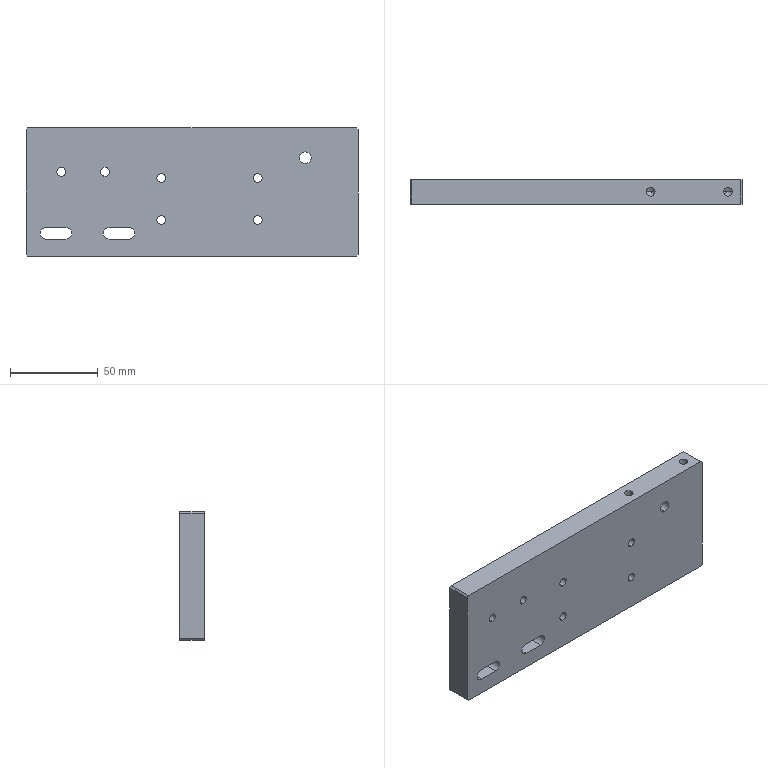Part | SolidWorks | features HoleWzd 5, Chamfer 1, Extrusion 1 | 1 solid | 43 faces | box 189 x 14 x 73 mm | volume 186915 mm3 | cylinder 24 | plane 15 | cone 4 | commonest cylinder face diameters 5 x16 6.6 x6 11 x2
STEP:
#1=CARTESIAN_POINT('',(64.5,0.2,14.));
#2=VERTEX_POINT('',#1);
#3=CARTESIAN_POINT('',(64.5,0.2,25.));
#4=VERTEX_POINT('',#3);
#5=CARTESIAN_POINT('',(64.5,0.2,19.5));
#6=DIRECTION('',(0.,1.,0.));
#7=DIRECTION('',(0.,0.,1.));
#8=AXIS2_PLACEMENT_3D('',#5,#6,#7);
#9=CIRCLE('',#8,5.5);
#10=EDGE_CURVE('',#2,#4,#9,.T.);
#11=ORIENTED_EDGE('',*,*,#10,.F.);
#12=CARTESIAN_POINT('',(64.5,7.,14.));
#13=VERTEX_POINT('',#12);
#14=CARTESIAN_POINT('',(64.5,7.,14.));
#15=DIRECTION('',(0.,1.,0.));
#16=VECTOR('',#15,1000.);
#17=LINE('',#14,#16);
#18=EDGE_CURVE('',#2,#13,#17,.T.);
#19=ORIENTED_EDGE('',*,*,#18,.T.);
#20=CARTESIAN_POINT('',(64.5,7.,25.));
#21=VERTEX_POINT('',#20);
#22=CARTESIAN_POINT('',(64.5,7.,19.5));
#23=DIRECTION('',(0.,1.,0.));
#24=DIRECTION('',(0.,0.,1.));
#25=AXIS2_PLACEMENT_3D('',#22,#23,#24);
#26=CIRCLE('',#25,5.5);
#27=EDGE_CURVE('',#13,#21,#26,.T.);
#28=ORIENTED_EDGE('',*,*,#27,.T.);
#29=CARTESIAN_POINT('',(64.5,7.,25.));
#30=DIRECTION('',(0.,1.,0.));
#31=VECTOR('',#30,1000.);
#32=LINE('',#29,#31);
#33=EDGE_CURVE('',#4,#21,#32,.T.);
#34=ORIENTED_EDGE('',*,*,#33,.F.);
#35=EDGE_LOOP('',(#11,#19,#28,#34));
#36=FACE_OUTER_BOUND('',#35,.T.);
#37=CARTESIAN_POINT('',(64.5,7.,19.5));
#38=DIRECTION('',(0.,1.,0.));
#39=DIRECTION('',(0.,0.,1.));
#40=AXIS2_PLACEMENT_3D('',#37,#38,#39);
#41=CYLINDRICAL_SURFACE('',#40,5.5);
#42=ADVANCED_FACE('',(#36),#41,.F.);
#43=CARTESIAN_POINT('',(64.5,-7.,16.2));
#44=VERTEX_POINT('',#43);
#45=CARTESIAN_POINT('',(64.5,-7.,22.8));
#46=VERTEX_POINT('',#45);
#47=CARTESIAN_POINT('',(64.5,-7.,19.5));
#48=DIRECTION('',(0.,1.,0.));
#49=DIRECTION('',(0.,0.,1.));
#50=AXIS2_PLACEMENT_3D('',#47,#48,#49);
#51=CIRCLE('',#50,3.3);
#52=EDGE_CURVE('',#44,#46,#51,.T.);
#53=ORIENTED_EDGE('',*,*,#52,.F.);
#54=CARTESIAN_POINT('',(64.5,0.2,16.2));
#55=VERTEX_POINT('',#54);
#56=CARTESIAN_POINT('',(64.5,7.,16.2));
#57=DIRECTION('',(0.,1.,0.));
#58=VECTOR('',#57,1000.);
#59=LINE('',#56,#58);
#60=EDGE_CURVE('',#44,#55,#59,.T.);
#61=ORIENTED_EDGE('',*,*,#60,.T.);
#62=CARTESIAN_POINT('',(64.5,0.2,22.8));
#63=VERTEX_POINT('',#62);
#64=CARTESIAN_POINT('',(64.5,0.2,19.5));
#65=DIRECTION('',(0.,1.,0.));
#66=DIRECTION('',(0.,0.,1.));
#67=AXIS2_PLACEMENT_3D('',#64,#65,#66);
#68=CIRCLE('',#67,3.3);
#69=EDGE_CURVE('',#55,#63,#68,.T.);
#70=ORIENTED_EDGE('',*,*,#69,.T.);
#71=CARTESIAN_POINT('',(64.5,7.,22.8));
#72=DIRECTION('',(0.,1.,0.));
#73=VECTOR('',#72,1000.);
#74=LINE('',#71,#73);
#75=EDGE_CURVE('',#46,#63,#74,.T.);
#76=ORIENTED_EDGE('',*,*,#75,.F.);
#77=EDGE_LOOP('',(#53,#61,#70,#76));
#78=FACE_OUTER_BOUND('',#77,.T.);
#79=CARTESIAN_POINT('',(64.5,7.,19.5));
#80=DIRECTION('',(0.,1.,0.));
#81=DIRECTION('',(0.,0.,1.));
#82=AXIS2_PLACEMENT_3D('',#79,#80,#81);
#83=CYLINDRICAL_SURFACE('',#82,3.3);
#84=ADVANCED_FACE('',(#78),#83,.F.);
#85=CARTESIAN_POINT('',(-74.5,-7.,9.));
#86=VERTEX_POINT('',#85);
#87=CARTESIAN_POINT('',(-74.5,-7.,14.));
#88=VERTEX_POINT('',#87);
#89=CARTESIAN_POINT('',(-74.5,-7.,11.5));
#90=DIRECTION('',(0.,1.,0.));
#91=DIRECTION('',(0.,0.,1.));
#92=AXIS2_PLACEMENT_3D('',#89,#90,#91);
#93=CIRCLE('',#92,2.5);
#94=EDGE_CURVE('',#86,#88,#93,.T.);
#95=ORIENTED_EDGE('',*,*,#94,.F.);
#96=CARTESIAN_POINT('',(-74.5,7.,9.));
#97=VERTEX_POINT('',#96);
#98=CARTESIAN_POINT('',(-74.5,7.,9.));
#99=DIRECTION('',(0.,1.,0.));
#100=VECTOR('',#99,1000.);
#101=LINE('',#98,#100);
#102=EDGE_CURVE('',#86,#97,#101,.T.);
#103=ORIENTED_EDGE('',*,*,#102,.T.);
#104=CARTESIAN_POINT('',(-74.5,7.,14.));
#105=VERTEX_POINT('',#104);
#106=CARTESIAN_POINT('',(-74.5,7.,11.5));
#107=DIRECTION('',(0.,1.,0.));
#108=DIRECTION('',(0.,0.,1.));
#109=AXIS2_PLACEMENT_3D('',#106,#107,#108);
#110=CIRCLE('',#109,2.5);
#111=EDGE_CURVE('',#97,#105,#110,.T.);
#112=ORIENTED_EDGE('',*,*,#111,.T.);
#113=CARTESIAN_POINT('',(-74.5,7.,14.));
#114=DIRECTION('',(0.,1.,0.));
#115=VECTOR('',#114,1000.);
#116=LINE('',#113,#115);
#117=EDGE_CURVE('',#88,#105,#116,.T.);
#118=ORIENTED_EDGE('',*,*,#117,.F.);
#119=EDGE_LOOP('',(#95,#103,#112,#118));
#120=FACE_OUTER_BOUND('',#119,.T.);
#121=CARTESIAN_POINT('',(-74.5,7.,11.5));
#122=DIRECTION('',(0.,1.,0.));
#123=DIRECTION('',(0.,0.,1.));
#124=AXIS2_PLACEMENT_3D('',#121,#122,#123);
#125=CYLINDRICAL_SURFACE('',#124,2.5);
#126=ADVANCED_FACE('',(#120),#125,.F.);
#127=CARTESIAN_POINT('',(-49.5,-7.,9.));
#128=VERTEX_POINT('',#127);
#129=CARTESIAN_POINT('',(-49.5,-7.,14.));
#130=VERTEX_POINT('',#129);
#131=CARTESIAN_POINT('',(-49.5,-7.,11.5));
#132=DIRECTION('',(0.,1.,0.));
#133=DIRECTION('',(0.,0.,1.));
#134=AXIS2_PLACEMENT_3D('',#131,#132,#133);
#135=CIRCLE('',#134,2.5);
#136=EDGE_CURVE('',#128,#130,#135,.T.);
#137=ORIENTED_EDGE('',*,*,#136,.F.);
#138=CARTESIAN_POINT('',(-49.5,7.,9.));
#139=VERTEX_POINT('',#138);
#140=CARTESIAN_POINT('',(-49.5,7.,9.));
#141=DIRECTION('',(0.,1.,0.));
#142=VECTOR('',#141,1000.);
#143=LINE('',#140,#142);
#144=EDGE_CURVE('',#128,#139,#143,.T.);
#145=ORIENTED_EDGE('',*,*,#144,.T.);
#146=CARTESIAN_POINT('',(-49.5,7.,14.));
#147=VERTEX_POINT('',#146);
#148=CARTESIAN_POINT('',(-49.5,7.,11.5));
#149=DIRECTION('',(0.,1.,0.));
#150=DIRECTION('',(0.,0.,1.));
#151=AXIS2_PLACEMENT_3D('',#148,#149,#150);
#152=CIRCLE('',#151,2.5);
#153=EDGE_CURVE('',#139,#147,#152,.T.);
#154=ORIENTED_EDGE('',*,*,#153,.T.);
#155=CARTESIAN_POINT('',(-49.5,7.,14.));
#156=DIRECTION('',(0.,1.,0.));
#157=VECTOR('',#156,1000.);
#158=LINE('',#155,#157);
#159=EDGE_CURVE('',#130,#147,#158,.T.);
#160=ORIENTED_EDGE('',*,*,#159,.F.);
#161=EDGE_LOOP('',(#137,#145,#154,#160));
#162=FACE_OUTER_BOUND('',#161,.T.);
#163=CARTESIAN_POINT('',(-49.5,7.,11.5));
#164=DIRECTION('',(0.,1.,0.));
#165=DIRECTION('',(0.,0.,1.));
#166=AXIS2_PLACEMENT_3D('',#163,#164,#165);
#167=CYLINDRICAL_SURFACE('',#166,2.5);
#168=ADVANCED_FACE('',(#162),#167,.F.);
#169=CARTESIAN_POINT('',(-17.5,-7.,-18.5));
#170=VERTEX_POINT('',#169);
#171=CARTESIAN_POINT('',(-17.5,-7.,-13.5));
#172=VERTEX_POINT('',#171);
#173=CARTESIAN_POINT('',(-17.5,-7.,-16.));
#174=DIRECTION('',(0.,1.,0.));
#175=DIRECTION('',(0.,0.,1.));
#176=AXIS2_PLACEMENT_3D('',#173,#174,#175);
#177=CIRCLE('',#176,2.5);
#178=EDGE_CURVE('',#170,#172,#177,.T.);
#179=ORIENTED_EDGE('',*,*,#178,.F.);
#180=CARTESIAN_POINT('',(-17.5,7.,-18.5));
#181=VERTEX_POINT('',#180);
#182=CARTESIAN_POINT('',(-17.5,7.,-18.5));
#183=DIRECTION('',(0.,1.,0.));
#184=VECTOR('',#183,1000.);
#185=LINE('',#182,#184);
#186=EDGE_CURVE('',#170,#181,#185,.T.);
#187=ORIENTED_EDGE('',*,*,#186,.T.);
#188=CARTESIAN_POINT('',(-17.5,7.,-13.5));
#189=VERTEX_POINT('',#188);
#190=CARTESIAN_POINT('',(-17.5,7.,-16.));
#191=DIRECTION('',(0.,1.,0.));
#192=DIRECTION('',(0.,0.,1.));
#193=AXIS2_PLACEMENT_3D('',#190,#191,#192);
#194=CIRCLE('',#193,2.5);
#195=EDGE_CURVE('',#181,#189,#194,.T.);
#196=ORIENTED_EDGE('',*,*,#195,.T.);
#197=CARTESIAN_POINT('',(-17.5,7.,-13.5));
#198=DIRECTION('',(0.,1.,0.));
#199=VECTOR('',#198,1000.);
#200=LINE('',#197,#199);
#201=EDGE_CURVE('',#172,#189,#200,.T.);
#202=ORIENTED_EDGE('',*,*,#201,.F.);
#203=EDGE_LOOP('',(#179,#187,#196,#202));
#204=FACE_OUTER_BOUND('',#203,.T.);
#205=CARTESIAN_POINT('',(-17.5,7.,-16.));
#206=DIRECTION('',(0.,1.,0.));
#207=DIRECTION('',(0.,0.,1.));
#208=AXIS2_PLACEMENT_3D('',#205,#206,#207);
#209=CYLINDRICAL_SURFACE('',#208,2.5);
#210=ADVANCED_FACE('',(#204),#209,.F.);
#211=CARTESIAN_POINT('',(37.5,-7.,5.5));
#212=VERTEX_POINT('',#211);
#213=CARTESIAN_POINT('',(37.5,-7.,10.5));
#214=VERTEX_POINT('',#213);
#215=CARTESIAN_POINT('',(37.5,-7.,8.));
#216=DIRECTION('',(0.,1.,0.));
#217=DIRECTION('',(0.,0.,1.));
#218=AXIS2_PLACEMENT_3D('',#215,#216,#217);
#219=CIRCLE('',#218,2.5);
#220=EDGE_CURVE('',#212,#214,#219,.T.);
#221=ORIENTED_EDGE('',*,*,#220,.F.);
#222=CARTESIAN_POINT('',(37.5,7.,5.5));
#223=VERTEX_POINT('',#222);
#224=CARTESIAN_POINT('',(37.5,7.,5.5));
#225=DIRECTION('',(0.,1.,0.));
#226=VECTOR('',#225,1000.);
#227=LINE('',#224,#226);
#228=EDGE_CURVE('',#212,#223,#227,.T.);
#229=ORIENTED_EDGE('',*,*,#228,.T.);
#230=CARTESIAN_POINT('',(37.5,7.,10.5));
#231=VERTEX_POINT('',#230);
#232=CARTESIAN_POINT('',(37.5,7.,8.));
#233=DIRECTION('',(0.,1.,0.));
#234=DIRECTION('',(0.,0.,1.));
#235=AXIS2_PLACEMENT_3D('',#232,#233,#234);
#236=CIRCLE('',#235,2.5);
#237=EDGE_CURVE('',#223,#231,#236,.T.);
#238=ORIENTED_EDGE('',*,*,#237,.T.);
#239=CARTESIAN_POINT('',(37.5,7.,10.5));
#240=DIRECTION('',(0.,1.,0.));
#241=VECTOR('',#240,1000.);
#242=LINE('',#239,#241);
#243=EDGE_CURVE('',#214,#231,#242,.T.);
#244=ORIENTED_EDGE('',*,*,#243,.F.);
#245=EDGE_LOOP('',(#221,#229,#238,#244));
#246=FACE_OUTER_BOUND('',#245,.T.);
#247=CARTESIAN_POINT('',(37.5,7.,8.));
#248=DIRECTION('',(0.,1.,0.));
#249=DIRECTION('',(0.,0.,1.));
#250=AXIS2_PLACEMENT_3D('',#247,#248,#249);
#251=CYLINDRICAL_SURFACE('',#250,2.5);
#252=ADVANCED_FACE('',(#246),#251,.F.);
#253=CARTESIAN_POINT('',(-17.5,-7.,5.5));
#254=VERTEX_POINT('',#253);
#255=CARTESIAN_POINT('',(-17.5,-7.,10.5));
#256=VERTEX_POINT('',#255);
#257=CARTESIAN_POINT('',(-17.5,-7.,8.));
#258=DIRECTION('',(0.,1.,0.));
#259=DIRECTION('',(0.,0.,1.));
#260=AXIS2_PLACEMENT_3D('',#257,#258,#259);
#261=CIRCLE('',#260,2.5);
#262=EDGE_CURVE('',#254,#256,#261,.T.);
#263=ORIENTED_EDGE('',*,*,#262,.F.);
#264=CARTESIAN_POINT('',(-17.5,7.,5.5));
#265=VERTEX_POINT('',#264);
#266=CARTESIAN_POINT('',(-17.5,7.,5.5));
#267=DIRECTION('',(0.,1.,0.));
#268=VECTOR('',#267,1000.);
#269=LINE('',#266,#268);
#270=EDGE_CURVE('',#254,#265,#269,.T.);
#271=ORIENTED_EDGE('',*,*,#270,.T.);
#272=CARTESIAN_POINT('',(-17.5,7.,10.5));
#273=VERTEX_POINT('',#272);
#274=CARTESIAN_POINT('',(-17.5,7.,8.));
#275=DIRECTION('',(0.,1.,0.));
#276=DIRECTION('',(0.,0.,1.));
#277=AXIS2_PLACEMENT_3D('',#274,#275,#276);
#278=CIRCLE('',#277,2.5);
#279=EDGE_CURVE('',#265,#273,#278,.T.);
#280=ORIENTED_EDGE('',*,*,#279,.T.);
#281=CARTESIAN_POINT('',(-17.5,7.,10.5));
#282=DIRECTION('',(0.,1.,0.));
#283=VECTOR('',#282,1000.);
#284=LINE('',#281,#283);
#285=EDGE_CURVE('',#256,#273,#284,.T.);
#286=ORIENTED_EDGE('',*,*,#285,.F.);
#287=EDGE_LOOP('',(#263,#271,#280,#286));
#288=FACE_OUTER_BOUND('',#287,.T.);
#289=CARTESIAN_POINT('',(-17.5,7.,8.));
#290=DIRECTION('',(0.,1.,0.));
#291=DIRECTION('',(0.,0.,1.));
#292=AXIS2_PLACEMENT_3D('',#289,#290,#291);
#293=CYLINDRICAL_SURFACE('',#292,2.5);
#294=ADVANCED_FACE('',(#288),#293,.F.);
#295=CARTESIAN_POINT('',(37.5,-7.,-18.5));
#296=VERTEX_POINT('',#295);
#297=CARTESIAN_POINT('',(37.5,-7.,-13.5));
#298=VERTEX_POINT('',#297);
#299=CARTESIAN_POINT('',(37.5,-7.,-16.));
#300=DIRECTION('',(0.,1.,0.));
#301=DIRECTION('',(0.,0.,1.));
#302=AXIS2_PLACEMENT_3D('',#299,#300,#301);
#303=CIRCLE('',#302,2.5);
#304=EDGE_CURVE('',#296,#298,#303,.T.);
#305=ORIENTED_EDGE('',*,*,#304,.F.);
#306=CARTESIAN_POINT('',(37.5,7.,-18.5));
#307=VERTEX_POINT('',#306);
#308=CARTESIAN_POINT('',(37.5,7.,-18.5));
#309=DIRECTION('',(0.,1.,0.));
#310=VECTOR('',#309,1000.);
#311=LINE('',#308,#310);
#312=EDGE_CURVE('',#296,#307,#311,.T.);
#313=ORIENTED_EDGE('',*,*,#312,.T.);
#314=CARTESIAN_POINT('',(37.5,7.,-13.5));
#315=VERTEX_POINT('',#314);
#316=CARTESIAN_POINT('',(37.5,7.,-16.));
#317=DIRECTION('',(0.,1.,0.));
#318=DIRECTION('',(0.,0.,1.));
#319=AXIS2_PLACEMENT_3D('',#316,#317,#318);
#320=CIRCLE('',#319,2.5);
#321=EDGE_CURVE('',#307,#315,#320,.T.);
#322=ORIENTED_EDGE('',*,*,#321,.T.);
#323=CARTESIAN_POINT('',(37.5,7.,-13.5));
#324=DIRECTION('',(0.,1.,0.));
#325=VECTOR('',#324,1000.);
#326=LINE('',#323,#325);
#327=EDGE_CURVE('',#298,#315,#326,.T.);
#328=ORIENTED_EDGE('',*,*,#327,.F.);
#329=EDGE_LOOP('',(#305,#313,#322,#328));
#330=FACE_OUTER_BOUND('',#329,.T.);
#331=CARTESIAN_POINT('',(37.5,7.,-16.));
#332=DIRECTION('',(0.,1.,0.));
#333=DIRECTION('',(0.,0.,1.));
#334=AXIS2_PLACEMENT_3D('',#331,#332,#333);
#335=CYLINDRICAL_SURFACE('',#334,2.5);
#336=ADVANCED_FACE('',(#330),#335,.F.);
#337=CARTESIAN_POINT('',(84.,0.,21.5));
#338=VERTEX_POINT('',#337);
#339=CARTESIAN_POINT('',(89.,0.,21.5));
#340=VERTEX_POINT('',#339);
#341=CARTESIAN_POINT('',(86.5,0.,21.5));
#342=DIRECTION('',(0.,0.,1.));
#343=DIRECTION('',(1.,0.,0.));
#344=AXIS2_PLACEMENT_3D('',#341,#342,#343);
#345=CIRCLE('',#344,2.5);
#346=EDGE_CURVE('',#338,#340,#345,.T.);
#347=ORIENTED_EDGE('',*,*,#346,.F.);
#348=CARTESIAN_POINT('',(84.,0.,36.5));
#349=VERTEX_POINT('',#348);
#350=CARTESIAN_POINT('',(84.,0.,36.5));
#351=DIRECTION('',(0.,0.,1.));
#352=VECTOR('',#351,1000.);
#353=LINE('',#350,#352);
#354=EDGE_CURVE('',#338,#349,#353,.T.);
#355=ORIENTED_EDGE('',*,*,#354,.T.);
#356=CARTESIAN_POINT('',(89.,0.,36.5));
#357=VERTEX_POINT('',#356);
#358=CARTESIAN_POINT('',(86.5,0.,36.5));
#359=DIRECTION('',(0.,0.,1.));
#360=DIRECTION('',(1.,0.,0.));
#361=AXIS2_PLACEMENT_3D('',#358,#359,#360);
#362=CIRCLE('',#361,2.5);
#363=EDGE_CURVE('',#349,#357,#362,.T.);
#364=ORIENTED_EDGE('',*,*,#363,.T.);
#365=CARTESIAN_POINT('',(89.,0.,36.5));
#366=DIRECTION('',(0.,0.,1.));
#367=VECTOR('',#366,1000.);
#368=LINE('',#365,#367);
#369=EDGE_CURVE('',#340,#357,#368,.T.);
#370=ORIENTED_EDGE('',*,*,#369,.F.);
#371=EDGE_LOOP('',(#347,#355,#364,#370));
#372=FACE_OUTER_BOUND('',#371,.T.);
#373=CARTESIAN_POINT('',(86.5,0.,36.5));
#374=DIRECTION('',(0.,0.,1.));
#375=DIRECTION('',(1.,0.,0.));
#376=AXIS2_PLACEMENT_3D('',#373,#374,#375);
#377=CYLINDRICAL_SURFACE('',#376,2.5);
#378=ADVANCED_FACE('',(#372),#377,.F.);
#379=CARTESIAN_POINT('',(86.5,0.,19.998));
#380=VERTEX_POINT('',#379);
#381=CARTESIAN_POINT('',(89.,0.,21.5));
#382=DIRECTION('',(0.8572,0.,0.515));
#383=VECTOR('',#382,1000.);
#384=LINE('',#381,#383);
#385=EDGE_CURVE('',#380,#340,#384,.T.);
#386=ORIENTED_EDGE('',*,*,#385,.F.);
#387=CARTESIAN_POINT('',(84.,0.,21.5));
#388=DIRECTION('',(-0.8572,0.,0.515));
#389=VECTOR('',#388,1000.);
#390=LINE('',#387,#389);
#391=EDGE_CURVE('',#380,#338,#390,.T.);
#392=ORIENTED_EDGE('',*,*,#391,.T.);
#393=ORIENTED_EDGE('',*,*,#346,.T.);
#394=EDGE_LOOP('',(#386,#392,#393));
#395=FACE_OUTER_BOUND('',#394,.T.);
#396=CARTESIAN_POINT('',(86.5,0.,21.5));
#397=DIRECTION('',(0.,0.,1.));
#398=DIRECTION('',(1.,0.,0.));
#399=AXIS2_PLACEMENT_3D('',#396,#397,#398);
#400=CONICAL_SURFACE('',#399,2.5,1.03);
#401=ADVANCED_FACE('',(#395),#400,.F.);
#402=CARTESIAN_POINT('',(40.,0.,21.5));
#403=VERTEX_POINT('',#402);
#404=CARTESIAN_POINT('',(45.,0.,21.5));
#405=VERTEX_POINT('',#404);
#406=CARTESIAN_POINT('',(42.5,0.,21.5));
#407=DIRECTION('',(0.,0.,1.));
#408=DIRECTION('',(1.,0.,0.));
#409=AXIS2_PLACEMENT_3D('',#406,#407,#408);
#410=CIRCLE('',#409,2.5);
#411=EDGE_CURVE('',#403,#405,#410,.T.);
#412=ORIENTED_EDGE('',*,*,#411,.F.);
#413=CARTESIAN_POINT('',(40.,0.,36.5));
#414=VERTEX_POINT('',#413);
#415=CARTESIAN_POINT('',(40.,0.,36.5));
#416=DIRECTION('',(0.,0.,1.));
#417=VECTOR('',#416,1000.);
#418=LINE('',#415,#417);
#419=EDGE_CURVE('',#403,#414,#418,.T.);
#420=ORIENTED_EDGE('',*,*,#419,.T.);
#421=CARTESIAN_POINT('',(45.,0.,36.5));
#422=VERTEX_POINT('',#421);
#423=CARTESIAN_POINT('',(42.5,0.,36.5));
#424=DIRECTION('',(0.,0.,1.));
#425=DIRECTION('',(1.,0.,0.));
#426=AXIS2_PLACEMENT_3D('',#423,#424,#425);
#427=CIRCLE('',#426,2.5);
#428=EDGE_CURVE('',#414,#422,#427,.T.);
#429=ORIENTED_EDGE('',*,*,#428,.T.);
#430=CARTESIAN_POINT('',(45.,0.,36.5));
#431=DIRECTION('',(0.,0.,1.));
#432=VECTOR('',#431,1000.);
#433=LINE('',#430,#432);
#434=EDGE_CURVE('',#405,#422,#433,.T.);
#435=ORIENTED_EDGE('',*,*,#434,.F.);
#436=EDGE_LOOP('',(#412,#420,#429,#435));
#437=FACE_OUTER_BOUND('',#436,.T.);
#438=CARTESIAN_POINT('',(42.5,0.,36.5));
#439=DIRECTION('',(0.,0.,1.));
#440=DIRECTION('',(1.,0.,0.));
#441=AXIS2_PLACEMENT_3D('',#438,#439,#440);
#442=CYLINDRICAL_SURFACE('',#441,2.5);
#443=ADVANCED_FACE('',(#437),#442,.F.);
#444=CARTESIAN_POINT('',(42.5,0.,19.998));
#445=VERTEX_POINT('',#444);
#446=CARTESIAN_POINT('',(45.,0.,21.5));
#447=DIRECTION('',(0.8572,0.,0.515));
#448=VECTOR('',#447,1000.);
#449=LINE('',#446,#448);
#450=EDGE_CURVE('',#445,#405,#449,.T.);
#451=ORIENTED_EDGE('',*,*,#450,.F.);
#452=CARTESIAN_POINT('',(40.,0.,21.5));
#453=DIRECTION('',(-0.8572,0.,0.515));
#454=VECTOR('',#453,1000.);
#455=LINE('',#452,#454);
#456=EDGE_CURVE('',#445,#403,#455,.T.);
#457=ORIENTED_EDGE('',*,*,#456,.T.);
#458=ORIENTED_EDGE('',*,*,#411,.T.);
#459=EDGE_LOOP('',(#451,#457,#458));
#460=FACE_OUTER_BOUND('',#459,.T.);
#461=CARTESIAN_POINT('',(42.5,0.,21.5));
#462=DIRECTION('',(0.,0.,1.));
#463=DIRECTION('',(1.,0.,0.));
#464=AXIS2_PLACEMENT_3D('',#461,#462,#463);
#465=CONICAL_SURFACE('',#464,2.5,1.03);
#466=ADVANCED_FACE('',(#460),#465,.F.);
#467=CARTESIAN_POINT('',(94.5,7.,35.5));
#468=VERTEX_POINT('',#467);
#469=CARTESIAN_POINT('',(94.5,7.,-35.5));
#470=VERTEX_POINT('',#469);
#471=CARTESIAN_POINT('',(94.5,7.,36.5));
#472=DIRECTION('',(0.,0.,-1.));
#473=VECTOR('',#472,1000.);
#474=LINE('',#471,#473);
#475=EDGE_CURVE('',#468,#470,#474,.T.);
#476=ORIENTED_EDGE('',*,*,#475,.F.);
#477=CARTESIAN_POINT('',(94.5,-7.,35.5));
#478=VERTEX_POINT('',#477);
#479=CARTESIAN_POINT('',(94.5,7.,35.5));
#480=DIRECTION('',(0.,-1.,0.));
#481=VECTOR('',#480,1000.);
#482=LINE('',#479,#481);
#483=EDGE_CURVE('',#468,#478,#482,.T.);
#484=ORIENTED_EDGE('',*,*,#483,.T.);
#485=CARTESIAN_POINT('',(94.5,-7.,-35.5));
#486=VERTEX_POINT('',#485);
#487=CARTESIAN_POINT('',(94.5,-7.,36.5));
#488=DIRECTION('',(0.,0.,-1.));
#489=VECTOR('',#488,1000.);
#490=LINE('',#487,#489);
#491=EDGE_CURVE('',#478,#486,#490,.T.);
#492=ORIENTED_EDGE('',*,*,#491,.T.);
#493=CARTESIAN_POINT('',(94.5,7.,-35.5));
#494=DIRECTION('',(0.,1.,0.));
#495=VECTOR('',#494,1000.);
#496=LINE('',#493,#495);
#497=EDGE_CURVE('',#486,#470,#496,.T.);
#498=ORIENTED_EDGE('',*,*,#497,.T.);
#499=EDGE_LOOP('',(#476,#484,#492,#498));
#500=FACE_OUTER_BOUND('',#499,.T.);
#501=CARTESIAN_POINT('',(94.5,7.,36.5));
#502=DIRECTION('',(-1.,0.,0.));
#503=DIRECTION('',(0.,0.,1.));
#504=AXIS2_PLACEMENT_3D('',#501,#502,#503);
#505=PLANE('',#504);
#506=ADVANCED_FACE('',(#500),#505,.F.);
#507=CARTESIAN_POINT('',(93.5,7.,-36.5));
#508=VERTEX_POINT('',#507);
#509=CARTESIAN_POINT('',(-93.5,7.,-36.5));
#510=VERTEX_POINT('',#509);
#511=CARTESIAN_POINT('',(-94.5,7.,-36.5));
#512=DIRECTION('',(-1.,0.,0.));
#513=VECTOR('',#512,1000.);
#514=LINE('',#511,#513);
#515=EDGE_CURVE('',#508,#510,#514,.T.);
#516=ORIENTED_EDGE('',*,*,#515,.F.);
#517=CARTESIAN_POINT('',(93.5,-7.,-36.5));
#518=VERTEX_POINT('',#517);
#519=CARTESIAN_POINT('',(93.5,7.,-36.5));
#520=DIRECTION('',(0.,-1.,0.));
#521=VECTOR('',#520,1000.);
#522=LINE('',#519,#521);
#523=EDGE_CURVE('',#508,#518,#522,.T.);
#524=ORIENTED_EDGE('',*,*,#523,.T.);
#525=CARTESIAN_POINT('',(-93.5,-7.,-36.5));
#526=VERTEX_POINT('',#525);
#527=CARTESIAN_POINT('',(-94.5,-7.,-36.5));
#528=DIRECTION('',(-1.,0.,0.));
#529=VECTOR('',#528,1000.);
#530=LINE('',#527,#529);
#531=EDGE_CURVE('',#518,#526,#530,.T.);
#532=ORIENTED_EDGE('',*,*,#531,.T.);
#533=CARTESIAN_POINT('',(-93.5,7.,-36.5));
#534=DIRECTION('',(0.,1.,0.));
#535=VECTOR('',#534,1000.);
#536=LINE('',#533,#535);
#537=EDGE_CURVE('',#526,#510,#536,.T.);
#538=ORIENTED_EDGE('',*,*,#537,.T.);
#539=EDGE_LOOP('',(#516,#524,#532,#538));
#540=FACE_OUTER_BOUND('',#539,.T.);
#541=CARTESIAN_POINT('',(-94.5,7.,-36.5));
#542=DIRECTION('',(0.,0.,1.));
#543=DIRECTION('',(1.,0.,0.));
#544=AXIS2_PLACEMENT_3D('',#541,#542,#543);
#545=PLANE('',#544);
#546=ADVANCED_FACE('',(#540),#545,.F.);
#547=CARTESIAN_POINT('',(-94.5,7.,-35.5));
#548=VERTEX_POINT('',#547);
#549=CARTESIAN_POINT('',(-94.5,7.,35.5));
#550=VERTEX_POINT('',#549);
#551=CARTESIAN_POINT('',(-94.5,7.,36.5));
#552=DIRECTION('',(0.,0.,1.));
#553=VECTOR('',#552,1000.);
#554=LINE('',#551,#553);
#555=EDGE_CURVE('',#548,#550,#554,.T.);
#556=ORIENTED_EDGE('',*,*,#555,.F.);
#557=CARTESIAN_POINT('',(-94.5,-7.,-35.5));
#558=VERTEX_POINT('',#557);
#559=CARTESIAN_POINT('',(-94.5,7.,-35.5));
#560=DIRECTION('',(0.,-1.,0.));
#561=VECTOR('',#560,1000.);
#562=LINE('',#559,#561);
#563=EDGE_CURVE('',#548,#558,#562,.T.);
#564=ORIENTED_EDGE('',*,*,#563,.T.);
#565=CARTESIAN_POINT('',(-94.5,-7.,35.5));
#566=VERTEX_POINT('',#565);
#567=CARTESIAN_POINT('',(-94.5,-7.,36.5));
#568=DIRECTION('',(0.,0.,1.));
#569=VECTOR('',#568,1000.);
#570=LINE('',#567,#569);
#571=EDGE_CURVE('',#558,#566,#570,.T.);
#572=ORIENTED_EDGE('',*,*,#571,.T.);
#573=CARTESIAN_POINT('',(-94.5,7.,35.5));
#574=DIRECTION('',(0.,1.,0.));
#575=VECTOR('',#574,1000.);
#576=LINE('',#573,#575);
#577=EDGE_CURVE('',#566,#550,#576,.T.);
#578=ORIENTED_EDGE('',*,*,#577,.T.);
#579=EDGE_LOOP('',(#556,#564,#572,#578));
#580=FACE_OUTER_BOUND('',#579,.T.);
#581=CARTESIAN_POINT('',(-94.5,7.,36.5));
#582=DIRECTION('',(1.,0.,0.));
#583=DIRECTION('',(0.,0.,-1.));
#584=AXIS2_PLACEMENT_3D('',#581,#582,#583);
#585=PLANE('',#584);
#586=ADVANCED_FACE('',(#580),#585,.F.);
#587=CARTESIAN_POINT('',(86.5,0.,36.5));
#588=DIRECTION('',(0.,0.,1.));
#589=DIRECTION('',(1.,0.,0.));
#590=AXIS2_PLACEMENT_3D('',#587,#588,#589);
#591=CIRCLE('',#590,2.5);
#592=EDGE_CURVE('',#357,#349,#591,.T.);
#593=ORIENTED_EDGE('',*,*,#592,.F.);
#594=ORIENTED_EDGE('',*,*,#363,.F.);
#595=EDGE_LOOP('',(#593,#594));
#596=FACE_BOUND('',#595,.T.);
#597=CARTESIAN_POINT('',(42.5,0.,36.5));
#598=DIRECTION('',(0.,0.,1.));
#599=DIRECTION('',(1.,0.,0.));
#600=AXIS2_PLACEMENT_3D('',#597,#598,#599);
#601=CIRCLE('',#600,2.5);
#602=EDGE_CURVE('',#422,#414,#601,.T.);
#603=ORIENTED_EDGE('',*,*,#602,.F.);
#604=ORIENTED_EDGE('',*,*,#428,.F.);
#605=EDGE_LOOP('',(#603,#604));
#606=FACE_BOUND('',#605,.T.);
#607=CARTESIAN_POINT('',(-93.5,-7.,36.5));
#608=VERTEX_POINT('',#607);
#609=CARTESIAN_POINT('',(93.5,-7.,36.5));
#610=VERTEX_POINT('',#609);
#611=CARTESIAN_POINT('',(-94.5,-7.,36.5));
#612=DIRECTION('',(1.,0.,0.));
#613=VECTOR('',#612,1000.);
#614=LINE('',#611,#613);
#615=EDGE_CURVE('',#608,#610,#614,.T.);
#616=ORIENTED_EDGE('',*,*,#615,.T.);
#617=CARTESIAN_POINT('',(93.5,7.,36.5));
#618=VERTEX_POINT('',#617);
#619=CARTESIAN_POINT('',(93.5,7.,36.5));
#620=DIRECTION('',(0.,1.,0.));
#621=VECTOR('',#620,1000.);
#622=LINE('',#619,#621);
#623=EDGE_CURVE('',#610,#618,#622,.T.);
#624=ORIENTED_EDGE('',*,*,#623,.T.);
#625=CARTESIAN_POINT('',(-93.5,7.,36.5));
#626=VERTEX_POINT('',#625);
#627=CARTESIAN_POINT('',(-94.5,7.,36.5));
#628=DIRECTION('',(1.,0.,0.));
#629=VECTOR('',#628,1000.);
#630=LINE('',#627,#629);
#631=EDGE_CURVE('',#626,#618,#630,.T.);
#632=ORIENTED_EDGE('',*,*,#631,.F.);
#633=CARTESIAN_POINT('',(-93.5,7.,36.5));
#634=DIRECTION('',(0.,-1.,0.));
#635=VECTOR('',#634,1000.);
#636=LINE('',#633,#635);
#637=EDGE_CURVE('',#626,#608,#636,.T.);
#638=ORIENTED_EDGE('',*,*,#637,.T.);
#639=EDGE_LOOP('',(#616,#624,#632,#638));
#640=FACE_OUTER_BOUND('',#639,.T.);
#641=CARTESIAN_POINT('',(-94.5,7.,36.5));
#642=DIRECTION('',(0.,0.,-1.));
#643=DIRECTION('',(-1.,0.,0.));
#644=AXIS2_PLACEMENT_3D('',#641,#642,#643);
#645=PLANE('',#644);
#646=ADVANCED_FACE('',(#596,#606,#640),#645,.F.);
#647=CARTESIAN_POINT('',(64.5,7.,19.5));
#648=DIRECTION('',(0.,1.,0.));
#649=DIRECTION('',(0.,0.,1.));
#650=AXIS2_PLACEMENT_3D('',#647,#648,#649);
#651=CIRCLE('',#650,5.5);
#652=EDGE_CURVE('',#21,#13,#651,.T.);
#653=ORIENTED_EDGE('',*,*,#652,.F.);
#654=ORIENTED_EDGE('',*,*,#27,.F.);
#655=EDGE_LOOP('',(#653,#654));
#656=FACE_BOUND('',#655,.T.);
#657=CARTESIAN_POINT('',(-74.5,7.,11.5));
#658=DIRECTION('',(0.,1.,0.));
#659=DIRECTION('',(0.,0.,1.));
#660=AXIS2_PLACEMENT_3D('',#657,#658,#659);
#661=CIRCLE('',#660,2.5);
#662=EDGE_CURVE('',#105,#97,#661,.T.);
#663=ORIENTED_EDGE('',*,*,#662,.F.);
#664=ORIENTED_EDGE('',*,*,#111,.F.);
#665=EDGE_LOOP('',(#663,#664));
#666=FACE_BOUND('',#665,.T.);
#667=CARTESIAN_POINT('',(-49.5,7.,11.5));
#668=DIRECTION('',(0.,1.,0.));
#669=DIRECTION('',(0.,0.,1.));
#670=AXIS2_PLACEMENT_3D('',#667,#668,#669);
#671=CIRCLE('',#670,2.5);
#672=EDGE_CURVE('',#147,#139,#671,.T.);
#673=ORIENTED_EDGE('',*,*,#672,.F.);
#674=ORIENTED_EDGE('',*,*,#153,.F.);
#675=EDGE_LOOP('',(#673,#674));
#676=FACE_BOUND('',#675,.T.);
#677=CARTESIAN_POINT('',(-83.2,7.,-20.2));
#678=VERTEX_POINT('',#677);
#679=CARTESIAN_POINT('',(-71.8,7.,-20.2));
#680=VERTEX_POINT('',#679);
#681=CARTESIAN_POINT('',(-83.2,7.,-20.2));
#682=DIRECTION('',(1.,0.,0.));
#683=VECTOR('',#682,1000.);
#684=LINE('',#681,#683);
#685=EDGE_CURVE('',#678,#680,#684,.T.);
#686=ORIENTED_EDGE('',*,*,#685,.F.);
#687=CARTESIAN_POINT('',(-83.2,7.,-26.8));
#688=VERTEX_POINT('',#687);
#689=CARTESIAN_POINT('',(-83.2,7.,-23.5));
#690=DIRECTION('',(0.,1.,0.));
#691=DIRECTION('',(0.,0.,1.));
#692=AXIS2_PLACEMENT_3D('',#689,#690,#691);
#693=CIRCLE('',#692,3.3);
#694=EDGE_CURVE('',#688,#678,#693,.T.);
#695=ORIENTED_EDGE('',*,*,#694,.F.);
#696=CARTESIAN_POINT('',(-71.8,7.,-26.8));
#697=VERTEX_POINT('',#696);
#698=CARTESIAN_POINT('',(-83.2,7.,-26.8));
#699=DIRECTION('',(1.,0.,0.));
#700=VECTOR('',#699,1000.);
#701=LINE('',#698,#700);
#702=EDGE_CURVE('',#688,#697,#701,.T.);
#703=ORIENTED_EDGE('',*,*,#702,.T.);
#704=CARTESIAN_POINT('',(-71.8,7.,-23.5));
#705=DIRECTION('',(0.,1.,0.));
#706=DIRECTION('',(0.,0.,1.));
#707=AXIS2_PLACEMENT_3D('',#704,#705,#706);
#708=CIRCLE('',#707,3.3);
#709=EDGE_CURVE('',#680,#697,#708,.T.);
#710=ORIENTED_EDGE('',*,*,#709,.F.);
#711=EDGE_LOOP('',(#686,#695,#703,#710));
#712=FACE_BOUND('',#711,.T.);
#713=CARTESIAN_POINT('',(-47.2,7.,-26.8));
#714=VERTEX_POINT('',#713);
#715=CARTESIAN_POINT('',(-47.2,7.,-20.2));
#716=VERTEX_POINT('',#715);
#717=CARTESIAN_POINT('',(-47.2,7.,-23.5));
#718=DIRECTION('',(0.,1.,0.));
#719=DIRECTION('',(0.,0.,1.));
#720=AXIS2_PLACEMENT_3D('',#717,#718,#719);
#721=CIRCLE('',#720,3.3);
#722=EDGE_CURVE('',#714,#716,#721,.T.);
#723=ORIENTED_EDGE('',*,*,#722,.F.);
#724=CARTESIAN_POINT('',(-35.8,7.,-26.8));
#725=VERTEX_POINT('',#724);
#726=CARTESIAN_POINT('',(-47.2,7.,-26.8));
#727=DIRECTION('',(1.,0.,0.));
#728=VECTOR('',#727,1000.);
#729=LINE('',#726,#728);
#730=EDGE_CURVE('',#714,#725,#729,.T.);
#731=ORIENTED_EDGE('',*,*,#730,.T.);
#732=CARTESIAN_POINT('',(-35.8,7.,-20.2));
#733=VERTEX_POINT('',#732);
#734=CARTESIAN_POINT('',(-35.8,7.,-23.5));
#735=DIRECTION('',(0.,1.,0.));
#736=DIRECTION('',(0.,0.,1.));
#737=AXIS2_PLACEMENT_3D('',#734,#735,#736);
#738=CIRCLE('',#737,3.3);
#739=EDGE_CURVE('',#733,#725,#738,.T.);
#740=ORIENTED_EDGE('',*,*,#739,.F.);
#741=CARTESIAN_POINT('',(-47.2,7.,-20.2));
#742=DIRECTION('',(1.,0.,0.));
#743=VECTOR('',#742,1000.);
#744=LINE('',#741,#743);
#745=EDGE_CURVE('',#716,#733,#744,.T.);
#746=ORIENTED_EDGE('',*,*,#745,.F.);
#747=EDGE_LOOP('',(#723,#731,#740,#746));
#748=FACE_BOUND('',#747,.T.);
#749=CARTESIAN_POINT('',(-17.5,7.,-16.));
#750=DIRECTION('',(0.,1.,0.));
#751=DIRECTION('',(0.,0.,1.));
#752=AXIS2_PLACEMENT_3D('',#749,#750,#751);
#753=CIRCLE('',#752,2.5);
#754=EDGE_CURVE('',#189,#181,#753,.T.);
#755=ORIENTED_EDGE('',*,*,#754,.F.);
#756=ORIENTED_EDGE('',*,*,#195,.F.);
#757=EDGE_LOOP('',(#755,#756));
#758=FACE_BOUND('',#757,.T.);
#759=CARTESIAN_POINT('',(37.5,7.,8.));
#760=DIRECTION('',(0.,1.,0.));
#761=DIRECTION('',(0.,0.,1.));
#762=AXIS2_PLACEMENT_3D('',#759,#760,#761);
#763=CIRCLE('',#762,2.5);
#764=EDGE_CURVE('',#231,#223,#763,.T.);
#765=ORIENTED_EDGE('',*,*,#764,.F.);
#766=ORIENTED_EDGE('',*,*,#237,.F.);
#767=EDGE_LOOP('',(#765,#766));
#768=FACE_BOUND('',#767,.T.);
#769=CARTESIAN_POINT('',(-17.5,7.,8.));
#770=DIRECTION('',(0.,1.,0.));
#771=DIRECTION('',(0.,0.,1.));
#772=AXIS2_PLACEMENT_3D('',#769,#770,#771);
#773=CIRCLE('',#772,2.5);
#774=EDGE_CURVE('',#273,#265,#773,.T.);
#775=ORIENTED_EDGE('',*,*,#774,.F.);
#776=ORIENTED_EDGE('',*,*,#279,.F.);
#777=EDGE_LOOP('',(#775,#776));
#778=FACE_BOUND('',#777,.T.);
#779=CARTESIAN_POINT('',(37.5,7.,-16.));
#780=DIRECTION('',(0.,1.,0.));
#781=DIRECTION('',(0.,0.,1.));
#782=AXIS2_PLACEMENT_3D('',#779,#780,#781);
#783=CIRCLE('',#782,2.5);
#784=EDGE_CURVE('',#315,#307,#783,.T.);
#785=ORIENTED_EDGE('',*,*,#784,.F.);
#786=ORIENTED_EDGE('',*,*,#321,.F.);
#787=EDGE_LOOP('',(#785,#786));
#788=FACE_BOUND('',#787,.T.);
#789=ORIENTED_EDGE('',*,*,#631,.T.);
#790=CARTESIAN_POINT('',(94.5,7.,35.5));
#791=DIRECTION('',(0.7071,0.,-0.7071));
#792=VECTOR('',#791,1000.);
#793=LINE('',#790,#792);
#794=EDGE_CURVE('',#618,#468,#793,.T.);
#795=ORIENTED_EDGE('',*,*,#794,.T.);
#796=ORIENTED_EDGE('',*,*,#475,.T.);
#797=CARTESIAN_POINT('',(93.5,7.,-36.5));
#798=DIRECTION('',(-0.7071,0.,-0.7071));
#799=VECTOR('',#798,1000.);
#800=LINE('',#797,#799);
#801=EDGE_CURVE('',#470,#508,#800,.T.);
#802=ORIENTED_EDGE('',*,*,#801,.T.);
#803=ORIENTED_EDGE('',*,*,#515,.T.);
#804=CARTESIAN_POINT('',(-94.5,7.,-35.5));
#805=DIRECTION('',(-0.7071,0.,0.7071));
#806=VECTOR('',#805,1000.);
#807=LINE('',#804,#806);
#808=EDGE_CURVE('',#510,#548,#807,.T.);
#809=ORIENTED_EDGE('',*,*,#808,.T.);
#810=ORIENTED_EDGE('',*,*,#555,.T.);
#811=CARTESIAN_POINT('',(-93.5,7.,36.5));
#812=DIRECTION('',(0.7071,0.,0.7071));
#813=VECTOR('',#812,1000.);
#814=LINE('',#811,#813);
#815=EDGE_CURVE('',#550,#626,#814,.T.);
#816=ORIENTED_EDGE('',*,*,#815,.T.);
#817=EDGE_LOOP('',(#789,#795,#796,#802,#803,#809,#810,#816));
#818=FACE_OUTER_BOUND('',#817,.T.);
#819=CARTESIAN_POINT('',(0.,7.,0.));
#820=DIRECTION('',(0.,-1.,0.));
#821=DIRECTION('',(0.,0.,-1.));
#822=AXIS2_PLACEMENT_3D('',#819,#820,#821);
#823=PLANE('',#822);
#824=ADVANCED_FACE('',(#656,#666,#676,#712,#748,#758,#768,#778,#788,#818),#823,.F.);
#825=CARTESIAN_POINT('',(64.5,-7.,19.5));
#826=DIRECTION('',(0.,1.,0.));
#827=DIRECTION('',(0.,0.,1.));
#828=AXIS2_PLACEMENT_3D('',#825,#826,#827);
#829=CIRCLE('',#828,3.3);
#830=EDGE_CURVE('',#46,#44,#829,.T.);
#831=ORIENTED_EDGE('',*,*,#830,.T.);
#832=ORIENTED_EDGE('',*,*,#52,.T.);
#833=EDGE_LOOP('',(#831,#832));
#834=FACE_BOUND('',#833,.T.);
#835=CARTESIAN_POINT('',(-74.5,-7.,11.5));
#836=DIRECTION('',(0.,1.,0.));
#837=DIRECTION('',(0.,0.,1.));
#838=AXIS2_PLACEMENT_3D('',#835,#836,#837);
#839=CIRCLE('',#838,2.5);
#840=EDGE_CURVE('',#88,#86,#839,.T.);
#841=ORIENTED_EDGE('',*,*,#840,.T.);
#842=ORIENTED_EDGE('',*,*,#94,.T.);
#843=EDGE_LOOP('',(#841,#842));
#844=FACE_BOUND('',#843,.T.);
#845=CARTESIAN_POINT('',(-49.5,-7.,11.5));
#846=DIRECTION('',(0.,1.,0.));
#847=DIRECTION('',(0.,0.,1.));
#848=AXIS2_PLACEMENT_3D('',#845,#846,#847);
#849=CIRCLE('',#848,2.5);
#850=EDGE_CURVE('',#130,#128,#849,.T.);
#851=ORIENTED_EDGE('',*,*,#850,.T.);
#852=ORIENTED_EDGE('',*,*,#136,.T.);
#853=EDGE_LOOP('',(#851,#852));
#854=FACE_BOUND('',#853,.T.);
#855=CARTESIAN_POINT('',(-83.2,-7.,-20.2));
#856=VERTEX_POINT('',#855);
#857=CARTESIAN_POINT('',(-71.8,-7.,-20.2));
#858=VERTEX_POINT('',#857);
#859=CARTESIAN_POINT('',(-83.2,-7.,-20.2));
#860=DIRECTION('',(1.,0.,0.));
#861=VECTOR('',#860,1000.);
#862=LINE('',#859,#861);
#863=EDGE_CURVE('',#856,#858,#862,.T.);
#864=ORIENTED_EDGE('',*,*,#863,.T.);
#865=CARTESIAN_POINT('',(-71.8,-7.,-26.8));
#866=VERTEX_POINT('',#865);
#867=CARTESIAN_POINT('',(-71.8,-7.,-23.5));
#868=DIRECTION('',(0.,1.,0.));
#869=DIRECTION('',(0.,0.,1.));
#870=AXIS2_PLACEMENT_3D('',#867,#868,#869);
#871=CIRCLE('',#870,3.3);
#872=EDGE_CURVE('',#858,#866,#871,.T.);
#873=ORIENTED_EDGE('',*,*,#872,.T.);
#874=CARTESIAN_POINT('',(-83.2,-7.,-26.8));
#875=VERTEX_POINT('',#874);
#876=CARTESIAN_POINT('',(-83.2,-7.,-26.8));
#877=DIRECTION('',(1.,0.,0.));
#878=VECTOR('',#877,1000.);
#879=LINE('',#876,#878);
#880=EDGE_CURVE('',#875,#866,#879,.T.);
#881=ORIENTED_EDGE('',*,*,#880,.F.);
#882=CARTESIAN_POINT('',(-83.2,-7.,-23.5));
#883=DIRECTION('',(0.,1.,0.));
#884=DIRECTION('',(0.,0.,1.));
#885=AXIS2_PLACEMENT_3D('',#882,#883,#884);
#886=CIRCLE('',#885,3.3);
#887=EDGE_CURVE('',#875,#856,#886,.T.);
#888=ORIENTED_EDGE('',*,*,#887,.T.);
#889=EDGE_LOOP('',(#864,#873,#881,#888));
#890=FACE_BOUND('',#889,.T.);
#891=CARTESIAN_POINT('',(-35.8,-7.,-20.2));
#892=VERTEX_POINT('',#891);
#893=CARTESIAN_POINT('',(-35.8,-7.,-26.8));
#894=VERTEX_POINT('',#893);
#895=CARTESIAN_POINT('',(-35.8,-7.,-23.5));
#896=DIRECTION('',(0.,1.,0.));
#897=DIRECTION('',(0.,0.,1.));
#898=AXIS2_PLACEMENT_3D('',#895,#896,#897);
#899=CIRCLE('',#898,3.3);
#900=EDGE_CURVE('',#892,#894,#899,.T.);
#901=ORIENTED_EDGE('',*,*,#900,.T.);
#902=CARTESIAN_POINT('',(-47.2,-7.,-26.8));
#903=VERTEX_POINT('',#902);
#904=CARTESIAN_POINT('',(-47.2,-7.,-26.8));
#905=DIRECTION('',(1.,0.,0.));
#906=VECTOR('',#905,1000.);
#907=LINE('',#904,#906);
#908=EDGE_CURVE('',#903,#894,#907,.T.);
#909=ORIENTED_EDGE('',*,*,#908,.F.);
#910=CARTESIAN_POINT('',(-47.2,-7.,-20.2));
#911=VERTEX_POINT('',#910);
#912=CARTESIAN_POINT('',(-47.2,-7.,-23.5));
#913=DIRECTION('',(0.,1.,0.));
#914=DIRECTION('',(0.,0.,1.));
#915=AXIS2_PLACEMENT_3D('',#912,#913,#914);
#916=CIRCLE('',#915,3.3);
#917=EDGE_CURVE('',#903,#911,#916,.T.);
#918=ORIENTED_EDGE('',*,*,#917,.T.);
#919=CARTESIAN_POINT('',(-47.2,-7.,-20.2));
#920=DIRECTION('',(1.,0.,0.));
#921=VECTOR('',#920,1000.);
#922=LINE('',#919,#921);
#923=EDGE_CURVE('',#911,#892,#922,.T.);
#924=ORIENTED_EDGE('',*,*,#923,.T.);
#925=EDGE_LOOP('',(#901,#909,#918,#924));
#926=FACE_BOUND('',#925,.T.);
#927=CARTESIAN_POINT('',(-17.5,-7.,-16.));
#928=DIRECTION('',(0.,1.,0.));
#929=DIRECTION('',(0.,0.,1.));
#930=AXIS2_PLACEMENT_3D('',#927,#928,#929);
#931=CIRCLE('',#930,2.5);
#932=EDGE_CURVE('',#172,#170,#931,.T.);
#933=ORIENTED_EDGE('',*,*,#932,.T.);
#934=ORIENTED_EDGE('',*,*,#178,.T.);
#935=EDGE_LOOP('',(#933,#934));
#936=FACE_BOUND('',#935,.T.);
#937=CARTESIAN_POINT('',(37.5,-7.,8.));
#938=DIRECTION('',(0.,1.,0.));
#939=DIRECTION('',(0.,0.,1.));
#940=AXIS2_PLACEMENT_3D('',#937,#938,#939);
#941=CIRCLE('',#940,2.5);
#942=EDGE_CURVE('',#214,#212,#941,.T.);
#943=ORIENTED_EDGE('',*,*,#942,.T.);
#944=ORIENTED_EDGE('',*,*,#220,.T.);
#945=EDGE_LOOP('',(#943,#944));
#946=FACE_BOUND('',#945,.T.);
#947=CARTESIAN_POINT('',(-17.5,-7.,8.));
#948=DIRECTION('',(0.,1.,0.));
#949=DIRECTION('',(0.,0.,1.));
#950=AXIS2_PLACEMENT_3D('',#947,#948,#949);
#951=CIRCLE('',#950,2.5);
#952=EDGE_CURVE('',#256,#254,#951,.T.);
#953=ORIENTED_EDGE('',*,*,#952,.T.);
#954=ORIENTED_EDGE('',*,*,#262,.T.);
#955=EDGE_LOOP('',(#953,#954));
#956=FACE_BOUND('',#955,.T.);
#957=CARTESIAN_POINT('',(37.5,-7.,-16.));
#958=DIRECTION('',(0.,1.,0.));
#959=DIRECTION('',(0.,0.,1.));
#960=AXIS2_PLACEMENT_3D('',#957,#958,#959);
#961=CIRCLE('',#960,2.5);
#962=EDGE_CURVE('',#298,#296,#961,.T.);
#963=ORIENTED_EDGE('',*,*,#962,.T.);
#964=ORIENTED_EDGE('',*,*,#304,.T.);
#965=EDGE_LOOP('',(#963,#964));
#966=FACE_BOUND('',#965,.T.);
#967=ORIENTED_EDGE('',*,*,#491,.F.);
#968=CARTESIAN_POINT('',(65.,-7.,65.));
#969=DIRECTION('',(-0.7071,0.,0.7071));
#970=VECTOR('',#969,1000.);
#971=LINE('',#968,#970);
#972=EDGE_CURVE('',#478,#610,#971,.T.);
#973=ORIENTED_EDGE('',*,*,#972,.T.);
#974=ORIENTED_EDGE('',*,*,#615,.F.);
#975=CARTESIAN_POINT('',(-65.,-7.,65.));
#976=DIRECTION('',(-0.7071,0.,-0.7071));
#977=VECTOR('',#976,1000.);
#978=LINE('',#975,#977);
#979=EDGE_CURVE('',#608,#566,#978,.T.);
#980=ORIENTED_EDGE('',*,*,#979,.T.);
#981=ORIENTED_EDGE('',*,*,#571,.F.);
#982=CARTESIAN_POINT('',(-65.,-7.,-65.));
#983=DIRECTION('',(0.7071,0.,-0.7071));
#984=VECTOR('',#983,1000.);
#985=LINE('',#982,#984);
#986=EDGE_CURVE('',#558,#526,#985,.T.);
#987=ORIENTED_EDGE('',*,*,#986,.T.);
#988=ORIENTED_EDGE('',*,*,#531,.F.);
#989=CARTESIAN_POINT('',(65.,-7.,-65.));
#990=DIRECTION('',(0.7071,0.,0.7071));
#991=VECTOR('',#990,1000.);
#992=LINE('',#989,#991);
#993=EDGE_CURVE('',#518,#486,#992,.T.);
#994=ORIENTED_EDGE('',*,*,#993,.T.);
#995=EDGE_LOOP('',(#967,#973,#974,#980,#981,#987,#988,#994));
#996=FACE_OUTER_BOUND('',#995,.T.);
#997=CARTESIAN_POINT('',(0.,-7.,0.));
#998=DIRECTION('',(0.,-1.,0.));
#999=DIRECTION('',(0.,0.,-1.));
#1000=AXIS2_PLACEMENT_3D('',#997,#998,#999);
#1001=PLANE('',#1000);
#1002=ADVANCED_FACE('',(#834,#844,#854,#890,#926,#936,#946,#956,#966,#996),#1001,.T.);
#1003=ORIENTED_EDGE('',*,*,#456,.F.);
#1004=ORIENTED_EDGE('',*,*,#450,.T.);
#1005=CARTESIAN_POINT('',(42.5,0.,21.5));
#1006=DIRECTION('',(0.,0.,1.));
#1007=DIRECTION('',(1.,0.,0.));
#1008=AXIS2_PLACEMENT_3D('',#1005,#1006,#1007);
#1009=CIRCLE('',#1008,2.5);
#1010=EDGE_CURVE('',#405,#403,#1009,.T.);
#1011=ORIENTED_EDGE('',*,*,#1010,.T.);
#1012=EDGE_LOOP('',(#1003,#1004,#1011));
#1013=FACE_OUTER_BOUND('',#1012,.T.);
#1014=CARTESIAN_POINT('',(42.5,0.,21.5));
#1015=DIRECTION('',(0.,0.,1.));
#1016=DIRECTION('',(1.,0.,0.));
#1017=AXIS2_PLACEMENT_3D('',#1014,#1015,#1016);
#1018=CONICAL_SURFACE('',#1017,2.5,1.03);
#1019=ADVANCED_FACE('',(#1013),#1018,.F.);
#1020=ORIENTED_EDGE('',*,*,#419,.F.);
#1021=ORIENTED_EDGE('',*,*,#1010,.F.);
#1022=ORIENTED_EDGE('',*,*,#434,.T.);
#1023=ORIENTED_EDGE('',*,*,#602,.T.);
#1024=EDGE_LOOP('',(#1020,#1021,#1022,#1023));
#1025=FACE_OUTER_BOUND('',#1024,.T.);
#1026=CARTESIAN_POINT('',(42.5,0.,36.5));
#1027=DIRECTION('',(0.,0.,1.));
#1028=DIRECTION('',(1.,0.,0.));
#1029=AXIS2_PLACEMENT_3D('',#1026,#1027,#1028);
#1030=CYLINDRICAL_SURFACE('',#1029,2.5);
#1031=ADVANCED_FACE('',(#1025),#1030,.F.);
#1032=ORIENTED_EDGE('',*,*,#391,.F.);
#1033=ORIENTED_EDGE('',*,*,#385,.T.);
#1034=CARTESIAN_POINT('',(86.5,0.,21.5));
#1035=DIRECTION('',(0.,0.,1.));
#1036=DIRECTION('',(1.,0.,0.));
#1037=AXIS2_PLACEMENT_3D('',#1034,#1035,#1036);
#1038=CIRCLE('',#1037,2.5);
#1039=EDGE_CURVE('',#340,#338,#1038,.T.);
#1040=ORIENTED_EDGE('',*,*,#1039,.T.);
#1041=EDGE_LOOP('',(#1032,#1033,#1040));
#1042=FACE_OUTER_BOUND('',#1041,.T.);
#1043=CARTESIAN_POINT('',(86.5,0.,21.5));
#1044=DIRECTION('',(0.,0.,1.));
#1045=DIRECTION('',(1.,0.,0.));
#1046=AXIS2_PLACEMENT_3D('',#1043,#1044,#1045);
#1047=CONICAL_SURFACE('',#1046,2.5,1.03);
#1048=ADVANCED_FACE('',(#1042),#1047,.F.);
#1049=ORIENTED_EDGE('',*,*,#354,.F.);
#1050=ORIENTED_EDGE('',*,*,#1039,.F.);
#1051=ORIENTED_EDGE('',*,*,#369,.T.);
#1052=ORIENTED_EDGE('',*,*,#592,.T.);
#1053=EDGE_LOOP('',(#1049,#1050,#1051,#1052));
#1054=FACE_OUTER_BOUND('',#1053,.T.);
#1055=CARTESIAN_POINT('',(86.5,0.,36.5));
#1056=DIRECTION('',(0.,0.,1.));
#1057=DIRECTION('',(1.,0.,0.));
#1058=AXIS2_PLACEMENT_3D('',#1055,#1056,#1057);
#1059=CYLINDRICAL_SURFACE('',#1058,2.5);
#1060=ADVANCED_FACE('',(#1054),#1059,.F.);
#1061=ORIENTED_EDGE('',*,*,#312,.F.);
#1062=ORIENTED_EDGE('',*,*,#962,.F.);
#1063=ORIENTED_EDGE('',*,*,#327,.T.);
#1064=ORIENTED_EDGE('',*,*,#784,.T.);
#1065=EDGE_LOOP('',(#1061,#1062,#1063,#1064));
#1066=FACE_OUTER_BOUND('',#1065,.T.);
#1067=CARTESIAN_POINT('',(37.5,7.,-16.));
#1068=DIRECTION('',(0.,1.,0.));
#1069=DIRECTION('',(0.,0.,1.));
#1070=AXIS2_PLACEMENT_3D('',#1067,#1068,#1069);
#1071=CYLINDRICAL_SURFACE('',#1070,2.5);
#1072=ADVANCED_FACE('',(#1066),#1071,.F.);
#1073=ORIENTED_EDGE('',*,*,#270,.F.);
#1074=ORIENTED_EDGE('',*,*,#952,.F.);
#1075=ORIENTED_EDGE('',*,*,#285,.T.);
#1076=ORIENTED_EDGE('',*,*,#774,.T.);
#1077=EDGE_LOOP('',(#1073,#1074,#1075,#1076));
#1078=FACE_OUTER_BOUND('',#1077,.T.);
#1079=CARTESIAN_POINT('',(-17.5,7.,8.));
#1080=DIRECTION('',(0.,1.,0.));
#1081=DIRECTION('',(0.,0.,1.));
#1082=AXIS2_PLACEMENT_3D('',#1079,#1080,#1081);
#1083=CYLINDRICAL_SURFACE('',#1082,2.5);
#1084=ADVANCED_FACE('',(#1078),#1083,.F.);
#1085=ORIENTED_EDGE('',*,*,#228,.F.);
#1086=ORIENTED_EDGE('',*,*,#942,.F.);
#1087=ORIENTED_EDGE('',*,*,#243,.T.);
#1088=ORIENTED_EDGE('',*,*,#764,.T.);
#1089=EDGE_LOOP('',(#1085,#1086,#1087,#1088));
#1090=FACE_OUTER_BOUND('',#1089,.T.);
#1091=CARTESIAN_POINT('',(37.5,7.,8.));
#1092=DIRECTION('',(0.,1.,0.));
#1093=DIRECTION('',(0.,0.,1.));
#1094=AXIS2_PLACEMENT_3D('',#1091,#1092,#1093);
#1095=CYLINDRICAL_SURFACE('',#1094,2.5);
#1096=ADVANCED_FACE('',(#1090),#1095,.F.);
#1097=ORIENTED_EDGE('',*,*,#186,.F.);
#1098=ORIENTED_EDGE('',*,*,#932,.F.);
#1099=ORIENTED_EDGE('',*,*,#201,.T.);
#1100=ORIENTED_EDGE('',*,*,#754,.T.);
#1101=EDGE_LOOP('',(#1097,#1098,#1099,#1100));
#1102=FACE_OUTER_BOUND('',#1101,.T.);
#1103=CARTESIAN_POINT('',(-17.5,7.,-16.));
#1104=DIRECTION('',(0.,1.,0.));
#1105=DIRECTION('',(0.,0.,1.));
#1106=AXIS2_PLACEMENT_3D('',#1103,#1104,#1105);
#1107=CYLINDRICAL_SURFACE('',#1106,2.5);
#1108=ADVANCED_FACE('',(#1102),#1107,.F.);
#1109=ORIENTED_EDGE('',*,*,#900,.F.);
#1110=CARTESIAN_POINT('',(-35.8,7.,-20.2));
#1111=DIRECTION('',(0.,-1.,0.));
#1112=VECTOR('',#1111,1000.);
#1113=LINE('',#1110,#1112);
#1114=EDGE_CURVE('',#733,#892,#1113,.T.);
#1115=ORIENTED_EDGE('',*,*,#1114,.F.);
#1116=ORIENTED_EDGE('',*,*,#739,.T.);
#1117=CARTESIAN_POINT('',(-35.8,7.,-26.8));
#1118=DIRECTION('',(0.,1.,0.));
#1119=VECTOR('',#1118,1000.);
#1120=LINE('',#1117,#1119);
#1121=EDGE_CURVE('',#894,#725,#1120,.T.);
#1122=ORIENTED_EDGE('',*,*,#1121,.F.);
#1123=EDGE_LOOP('',(#1109,#1115,#1116,#1122));
#1124=FACE_OUTER_BOUND('',#1123,.T.);
#1125=CARTESIAN_POINT('',(-35.8,7.,-23.5));
#1126=DIRECTION('',(0.,1.,0.));
#1127=DIRECTION('',(0.,0.,1.));
#1128=AXIS2_PLACEMENT_3D('',#1125,#1126,#1127);
#1129=CYLINDRICAL_SURFACE('',#1128,3.3);
#1130=ADVANCED_FACE('',(#1124),#1129,.F.);
#1131=ORIENTED_EDGE('',*,*,#722,.T.);
#1132=CARTESIAN_POINT('',(-47.2,7.,-20.2));
#1133=DIRECTION('',(0.,1.,0.));
#1134=VECTOR('',#1133,1000.);
#1135=LINE('',#1132,#1134);
#1136=EDGE_CURVE('',#911,#716,#1135,.T.);
#1137=ORIENTED_EDGE('',*,*,#1136,.F.);
#1138=ORIENTED_EDGE('',*,*,#917,.F.);
#1139=CARTESIAN_POINT('',(-47.2,7.,-26.8));
#1140=DIRECTION('',(0.,-1.,0.));
#1141=VECTOR('',#1140,1000.);
#1142=LINE('',#1139,#1141);
#1143=EDGE_CURVE('',#714,#903,#1142,.T.);
#1144=ORIENTED_EDGE('',*,*,#1143,.F.);
#1145=EDGE_LOOP('',(#1131,#1137,#1138,#1144));
#1146=FACE_OUTER_BOUND('',#1145,.T.);
#1147=CARTESIAN_POINT('',(-47.2,7.,-23.5));
#1148=DIRECTION('',(0.,1.,0.));
#1149=DIRECTION('',(0.,0.,1.));
#1150=AXIS2_PLACEMENT_3D('',#1147,#1148,#1149);
#1151=CYLINDRICAL_SURFACE('',#1150,3.3);
#1152=ADVANCED_FACE('',(#1146),#1151,.F.);
#1153=ORIENTED_EDGE('',*,*,#1121,.T.);
#1154=ORIENTED_EDGE('',*,*,#730,.F.);
#1155=ORIENTED_EDGE('',*,*,#1143,.T.);
#1156=ORIENTED_EDGE('',*,*,#908,.T.);
#1157=EDGE_LOOP('',(#1153,#1154,#1155,#1156));
#1158=FACE_OUTER_BOUND('',#1157,.T.);
#1159=CARTESIAN_POINT('',(-47.2,7.,-26.8));
#1160=DIRECTION('',(0.,0.,-1.));
#1161=DIRECTION('',(-1.,0.,0.));
#1162=AXIS2_PLACEMENT_3D('',#1159,#1160,#1161);
#1163=PLANE('',#1162);
#1164=ADVANCED_FACE('',(#1158),#1163,.F.);
#1165=ORIENTED_EDGE('',*,*,#1114,.T.);
#1166=ORIENTED_EDGE('',*,*,#923,.F.);
#1167=ORIENTED_EDGE('',*,*,#1136,.T.);
#1168=ORIENTED_EDGE('',*,*,#745,.T.);
#1169=EDGE_LOOP('',(#1165,#1166,#1167,#1168));
#1170=FACE_OUTER_BOUND('',#1169,.T.);
#1171=CARTESIAN_POINT('',(-47.2,7.,-20.2));
#1172=DIRECTION('',(0.,0.,1.));
#1173=DIRECTION('',(1.,0.,0.));
#1174=AXIS2_PLACEMENT_3D('',#1171,#1172,#1173);
#1175=PLANE('',#1174);
#1176=ADVANCED_FACE('',(#1170),#1175,.F.);
#1177=ORIENTED_EDGE('',*,*,#872,.F.);
#1178=CARTESIAN_POINT('',(-71.8,7.,-20.2));
#1179=DIRECTION('',(0.,-1.,0.));
#1180=VECTOR('',#1179,1000.);
#1181=LINE('',#1178,#1180);
#1182=EDGE_CURVE('',#680,#858,#1181,.T.);
#1183=ORIENTED_EDGE('',*,*,#1182,.F.);
#1184=ORIENTED_EDGE('',*,*,#709,.T.);
#1185=CARTESIAN_POINT('',(-71.8,7.,-26.8));
#1186=DIRECTION('',(0.,1.,0.));
#1187=VECTOR('',#1186,1000.);
#1188=LINE('',#1185,#1187);
#1189=EDGE_CURVE('',#866,#697,#1188,.T.);
#1190=ORIENTED_EDGE('',*,*,#1189,.F.);
#1191=EDGE_LOOP('',(#1177,#1183,#1184,#1190));
#1192=FACE_OUTER_BOUND('',#1191,.T.);
#1193=CARTESIAN_POINT('',(-71.8,7.,-23.5));
#1194=DIRECTION('',(0.,1.,0.));
#1195=DIRECTION('',(0.,0.,1.));
#1196=AXIS2_PLACEMENT_3D('',#1193,#1194,#1195);
#1197=CYLINDRICAL_SURFACE('',#1196,3.3);
#1198=ADVANCED_FACE('',(#1192),#1197,.F.);
#1199=ORIENTED_EDGE('',*,*,#694,.T.);
#1200=CARTESIAN_POINT('',(-83.2,7.,-20.2));
#1201=DIRECTION('',(0.,1.,0.));
#1202=VECTOR('',#1201,1000.);
#1203=LINE('',#1200,#1202);
#1204=EDGE_CURVE('',#856,#678,#1203,.T.);
#1205=ORIENTED_EDGE('',*,*,#1204,.F.);
#1206=ORIENTED_EDGE('',*,*,#887,.F.);
#1207=CARTESIAN_POINT('',(-83.2,7.,-26.8));
#1208=DIRECTION('',(0.,-1.,0.));
#1209=VECTOR('',#1208,1000.);
#1210=LINE('',#1207,#1209);
#1211=EDGE_CURVE('',#688,#875,#1210,.T.);
#1212=ORIENTED_EDGE('',*,*,#1211,.F.);
#1213=EDGE_LOOP('',(#1199,#1205,#1206,#1212));
#1214=FACE_OUTER_BOUND('',#1213,.T.);
#1215=CARTESIAN_POINT('',(-83.2,7.,-23.5));
#1216=DIRECTION('',(0.,1.,0.));
#1217=DIRECTION('',(0.,0.,1.));
#1218=AXIS2_PLACEMENT_3D('',#1215,#1216,#1217);
#1219=CYLINDRICAL_SURFACE('',#1218,3.3);
#1220=ADVANCED_FACE('',(#1214),#1219,.F.);
#1221=ORIENTED_EDGE('',*,*,#1189,.T.);
#1222=ORIENTED_EDGE('',*,*,#702,.F.);
#1223=ORIENTED_EDGE('',*,*,#1211,.T.);
#1224=ORIENTED_EDGE('',*,*,#880,.T.);
#1225=EDGE_LOOP('',(#1221,#1222,#1223,#1224));
#1226=FACE_OUTER_BOUND('',#1225,.T.);
#1227=CARTESIAN_POINT('',(-83.2,7.,-26.8));
#1228=DIRECTION('',(0.,0.,-1.));
#1229=DIRECTION('',(-1.,0.,0.));
#1230=AXIS2_PLACEMENT_3D('',#1227,#1228,#1229);
#1231=PLANE('',#1230);
#1232=ADVANCED_FACE('',(#1226),#1231,.F.);
#1233=ORIENTED_EDGE('',*,*,#1182,.T.);
#1234=ORIENTED_EDGE('',*,*,#863,.F.);
#1235=ORIENTED_EDGE('',*,*,#1204,.T.);
#1236=ORIENTED_EDGE('',*,*,#685,.T.);
#1237=EDGE_LOOP('',(#1233,#1234,#1235,#1236));
#1238=FACE_OUTER_BOUND('',#1237,.T.);
#1239=CARTESIAN_POINT('',(-83.2,7.,-20.2));
#1240=DIRECTION('',(0.,0.,1.));
#1241=DIRECTION('',(1.,0.,0.));
#1242=AXIS2_PLACEMENT_3D('',#1239,#1240,#1241);
#1243=PLANE('',#1242);
#1244=ADVANCED_FACE('',(#1238),#1243,.F.);
#1245=ORIENTED_EDGE('',*,*,#144,.F.);
#1246=ORIENTED_EDGE('',*,*,#850,.F.);
#1247=ORIENTED_EDGE('',*,*,#159,.T.);
#1248=ORIENTED_EDGE('',*,*,#672,.T.);
#1249=EDGE_LOOP('',(#1245,#1246,#1247,#1248));
#1250=FACE_OUTER_BOUND('',#1249,.T.);
#1251=CARTESIAN_POINT('',(-49.5,7.,11.5));
#1252=DIRECTION('',(0.,1.,0.));
#1253=DIRECTION('',(0.,0.,1.));
#1254=AXIS2_PLACEMENT_3D('',#1251,#1252,#1253);
#1255=CYLINDRICAL_SURFACE('',#1254,2.5);
#1256=ADVANCED_FACE('',(#1250),#1255,.F.);
#1257=ORIENTED_EDGE('',*,*,#102,.F.);
#1258=ORIENTED_EDGE('',*,*,#840,.F.);
#1259=ORIENTED_EDGE('',*,*,#117,.T.);
#1260=ORIENTED_EDGE('',*,*,#662,.T.);
#1261=EDGE_LOOP('',(#1257,#1258,#1259,#1260));
#1262=FACE_OUTER_BOUND('',#1261,.T.);
#1263=CARTESIAN_POINT('',(-74.5,7.,11.5));
#1264=DIRECTION('',(0.,1.,0.));
#1265=DIRECTION('',(0.,0.,1.));
#1266=AXIS2_PLACEMENT_3D('',#1263,#1264,#1265);
#1267=CYLINDRICAL_SURFACE('',#1266,2.5);
#1268=ADVANCED_FACE('',(#1262),#1267,.F.);
#1269=ORIENTED_EDGE('',*,*,#794,.F.);
#1270=ORIENTED_EDGE('',*,*,#623,.F.);
#1271=ORIENTED_EDGE('',*,*,#972,.F.);
#1272=ORIENTED_EDGE('',*,*,#483,.F.);
#1273=EDGE_LOOP('',(#1269,#1270,#1271,#1272));
#1274=FACE_OUTER_BOUND('',#1273,.T.);
#1275=CARTESIAN_POINT('',(94.5,7.,35.5));
#1276=DIRECTION('',(-0.7071,0.,-0.7071));
#1277=DIRECTION('',(0.,-1.,0.));
#1278=AXIS2_PLACEMENT_3D('',#1275,#1276,#1277);
#1279=PLANE('',#1278);
#1280=ADVANCED_FACE('',(#1274),#1279,.F.);
#1281=ORIENTED_EDGE('',*,*,#801,.F.);
#1282=ORIENTED_EDGE('',*,*,#497,.F.);
#1283=ORIENTED_EDGE('',*,*,#993,.F.);
#1284=ORIENTED_EDGE('',*,*,#523,.F.);
#1285=EDGE_LOOP('',(#1281,#1282,#1283,#1284));
#1286=FACE_OUTER_BOUND('',#1285,.T.);
#1287=CARTESIAN_POINT('',(93.5,7.,-36.5));
#1288=DIRECTION('',(-0.7071,0.,0.7071));
#1289=DIRECTION('',(0.,-1.,0.));
#1290=AXIS2_PLACEMENT_3D('',#1287,#1288,#1289);
#1291=PLANE('',#1290);
#1292=ADVANCED_FACE('',(#1286),#1291,.F.);
#1293=ORIENTED_EDGE('',*,*,#808,.F.);
#1294=ORIENTED_EDGE('',*,*,#537,.F.);
#1295=ORIENTED_EDGE('',*,*,#986,.F.);
#1296=ORIENTED_EDGE('',*,*,#563,.F.);
#1297=EDGE_LOOP('',(#1293,#1294,#1295,#1296));
#1298=FACE_OUTER_BOUND('',#1297,.T.);
#1299=CARTESIAN_POINT('',(-94.5,7.,-35.5));
#1300=DIRECTION('',(0.7071,0.,0.7071));
#1301=DIRECTION('',(0.,-1.,0.));
#1302=AXIS2_PLACEMENT_3D('',#1299,#1300,#1301);
#1303=PLANE('',#1302);
#1304=ADVANCED_FACE('',(#1298),#1303,.F.);
#1305=ORIENTED_EDGE('',*,*,#815,.F.);
#1306=ORIENTED_EDGE('',*,*,#577,.F.);
#1307=ORIENTED_EDGE('',*,*,#979,.F.);
#1308=ORIENTED_EDGE('',*,*,#637,.F.);
#1309=EDGE_LOOP('',(#1305,#1306,#1307,#1308));
#1310=FACE_OUTER_BOUND('',#1309,.T.);
#1311=CARTESIAN_POINT('',(-93.5,7.,36.5));
#1312=DIRECTION('',(0.7071,0.,-0.7071));
#1313=DIRECTION('',(0.,-1.,0.));
#1314=AXIS2_PLACEMENT_3D('',#1311,#1312,#1313);
#1315=PLANE('',#1314);
#1316=ADVANCED_FACE('',(#1310),#1315,.F.);
#1317=ORIENTED_EDGE('',*,*,#60,.F.);
#1318=ORIENTED_EDGE('',*,*,#830,.F.);
#1319=ORIENTED_EDGE('',*,*,#75,.T.);
#1320=CARTESIAN_POINT('',(64.5,0.2,19.5));
#1321=DIRECTION('',(0.,1.,0.));
#1322=DIRECTION('',(0.,0.,1.));
#1323=AXIS2_PLACEMENT_3D('',#1320,#1321,#1322);
#1324=CIRCLE('',#1323,3.3);
#1325=EDGE_CURVE('',#63,#55,#1324,.T.);
#1326=ORIENTED_EDGE('',*,*,#1325,.T.);
#1327=EDGE_LOOP('',(#1317,#1318,#1319,#1326));
#1328=FACE_OUTER_BOUND('',#1327,.T.);
#1329=CARTESIAN_POINT('',(64.5,7.,19.5));
#1330=DIRECTION('',(0.,1.,0.));
#1331=DIRECTION('',(0.,0.,1.));
#1332=AXIS2_PLACEMENT_3D('',#1329,#1330,#1331);
#1333=CYLINDRICAL_SURFACE('',#1332,3.3);
#1334=ADVANCED_FACE('',(#1328),#1333,.F.);
#1335=ORIENTED_EDGE('',*,*,#1325,.F.);
#1336=ORIENTED_EDGE('',*,*,#69,.F.);
#1337=EDGE_LOOP('',(#1335,#1336));
#1338=FACE_BOUND('',#1337,.T.);
#1339=CARTESIAN_POINT('',(64.5,0.2,19.5));
#1340=DIRECTION('',(0.,1.,0.));
#1341=DIRECTION('',(0.,0.,1.));
#1342=AXIS2_PLACEMENT_3D('',#1339,#1340,#1341);
#1343=CIRCLE('',#1342,5.5);
#1344=EDGE_CURVE('',#4,#2,#1343,.T.);
#1345=ORIENTED_EDGE('',*,*,#1344,.T.);
#1346=ORIENTED_EDGE('',*,*,#10,.T.);
#1347=EDGE_LOOP('',(#1345,#1346));
#1348=FACE_OUTER_BOUND('',#1347,.T.);
#1349=CARTESIAN_POINT('',(67.8,0.2,19.5));
#1350=DIRECTION('',(0.,-1.,0.));
#1351=DIRECTION('',(0.,0.,-1.));
#1352=AXIS2_PLACEMENT_3D('',#1349,#1350,#1351);
#1353=PLANE('',#1352);
#1354=ADVANCED_FACE('',(#1338,#1348),#1353,.F.);
#1355=ORIENTED_EDGE('',*,*,#18,.F.);
#1356=ORIENTED_EDGE('',*,*,#1344,.F.);
#1357=ORIENTED_EDGE('',*,*,#33,.T.);
#1358=ORIENTED_EDGE('',*,*,#652,.T.);
#1359=EDGE_LOOP('',(#1355,#1356,#1357,#1358));
#1360=FACE_OUTER_BOUND('',#1359,.T.);
#1361=CARTESIAN_POINT('',(64.5,7.,19.5));
#1362=DIRECTION('',(0.,1.,0.));
#1363=DIRECTION('',(0.,0.,1.));
#1364=AXIS2_PLACEMENT_3D('',#1361,#1362,#1363);
#1365=CYLINDRICAL_SURFACE('',#1364,5.5);
#1366=ADVANCED_FACE('',(#1360),#1365,.F.);
#1367=CLOSED_SHELL('',(#42,#84,#126,#168,#210,#252,#294,#336,#378,#401,#443,#466,#506,#546,#586,#646,#824,#1002,#1019,#1031,#1048,#1060,#1072,#1084,#1096,#1108,#1130,#1152,#1164,#1176,#1198,#1220,#1232,#1244,#1256,#1268,#1280,#1292,#1304,#1316,#1334,#1354,#1366));
#1368=MANIFOLD_SOLID_BREP('',#1367);
#1369=CARTESIAN_POINT('',(0.,0.,0.));
#1370=DIRECTION('',(0.,0.,1.));
#1371=DIRECTION('',(1.,0.,0.));
#1372=AXIS2_PLACEMENT_3D('',#1369,#1370,#1371);
#1373=(LENGTH_UNIT()NAMED_UNIT(*)SI_UNIT(.MILLI.,.METRE.));
#1374=UNCERTAINTY_MEASURE_WITH_UNIT(LENGTH_MEASURE(0.00001),#1373,'','');
#1375=(NAMED_UNIT(*)PLANE_ANGLE_UNIT()SI_UNIT($,.RADIAN.));
#1376=(NAMED_UNIT(*)SI_UNIT($,.STERADIAN.)SOLID_ANGLE_UNIT());
#1377=(GEOMETRIC_REPRESENTATION_CONTEXT(3)GLOBAL_UNCERTAINTY_ASSIGNED_CONTEXT((#1374))GLOBAL_UNIT_ASSIGNED_CONTEXT((#1373,#1375,#1376))REPRESENTATION_CONTEXT('',''));
#1378=ADVANCED_BREP_SHAPE_REPRESENTATION('',(#1368,#1372),#1377);